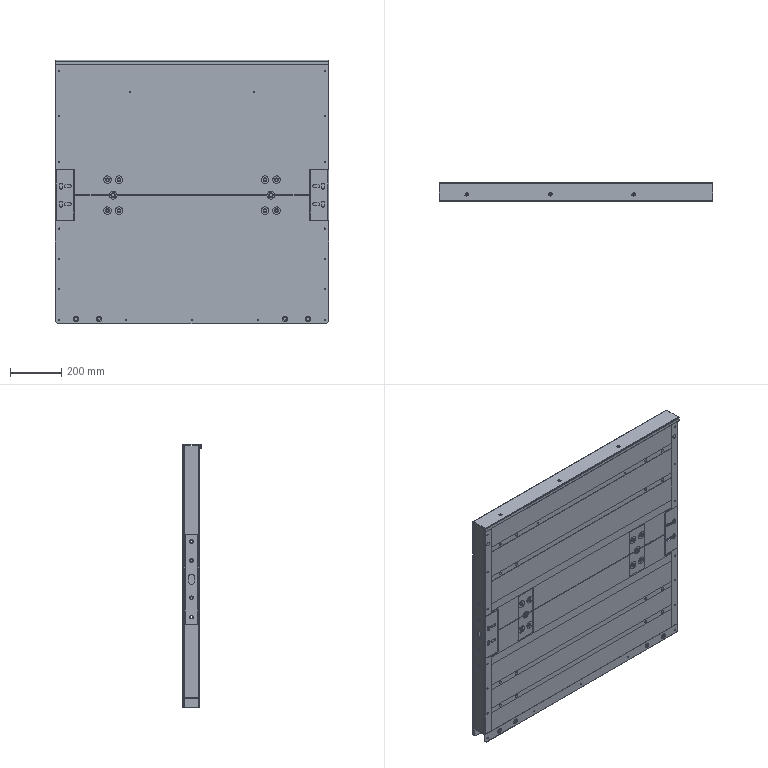Part | 50 solids | 1658 faces | box 1064 x 72 x 1025 mm | volume 8869171 mm3 | plane 924 | cylinder 590 | cone 144 | commonest cylinder face diameters 10 x86 11 x80 14.5 x48 5 x34 14.75 x32 15.07 x32